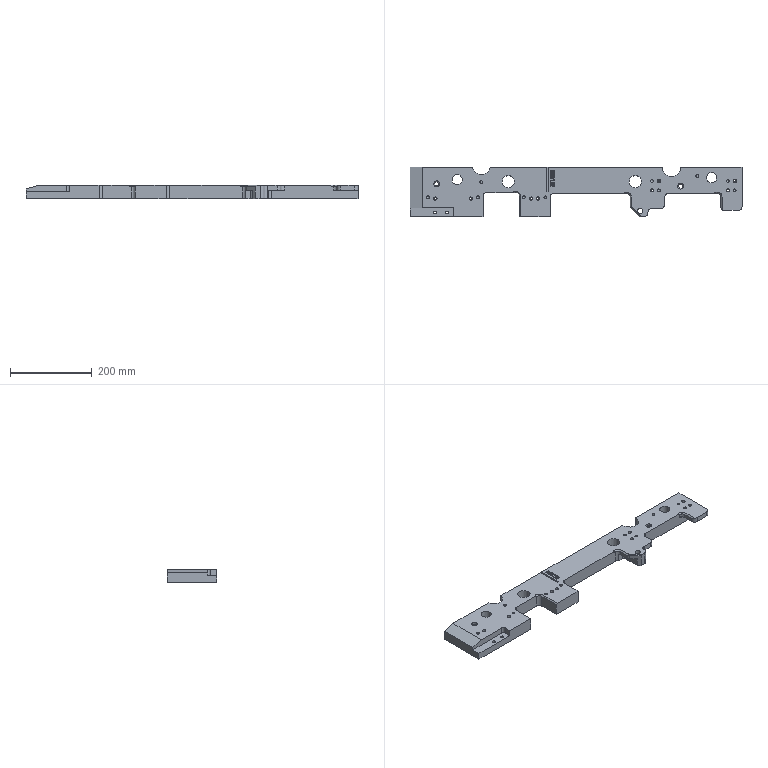Part | STEP file | gslz 2016.10.28-13_id1566_x_t | 1 solid | 224 faces | box 810 x 120 x 32 mm | volume 2005033 mm3 | plane 127 | cylinder 62 | cone 22 | other 13 | commonest cylinder face diameters 6.8 x16 18 x12 8 x9 6 x8 5.2 x4 10.3 x2